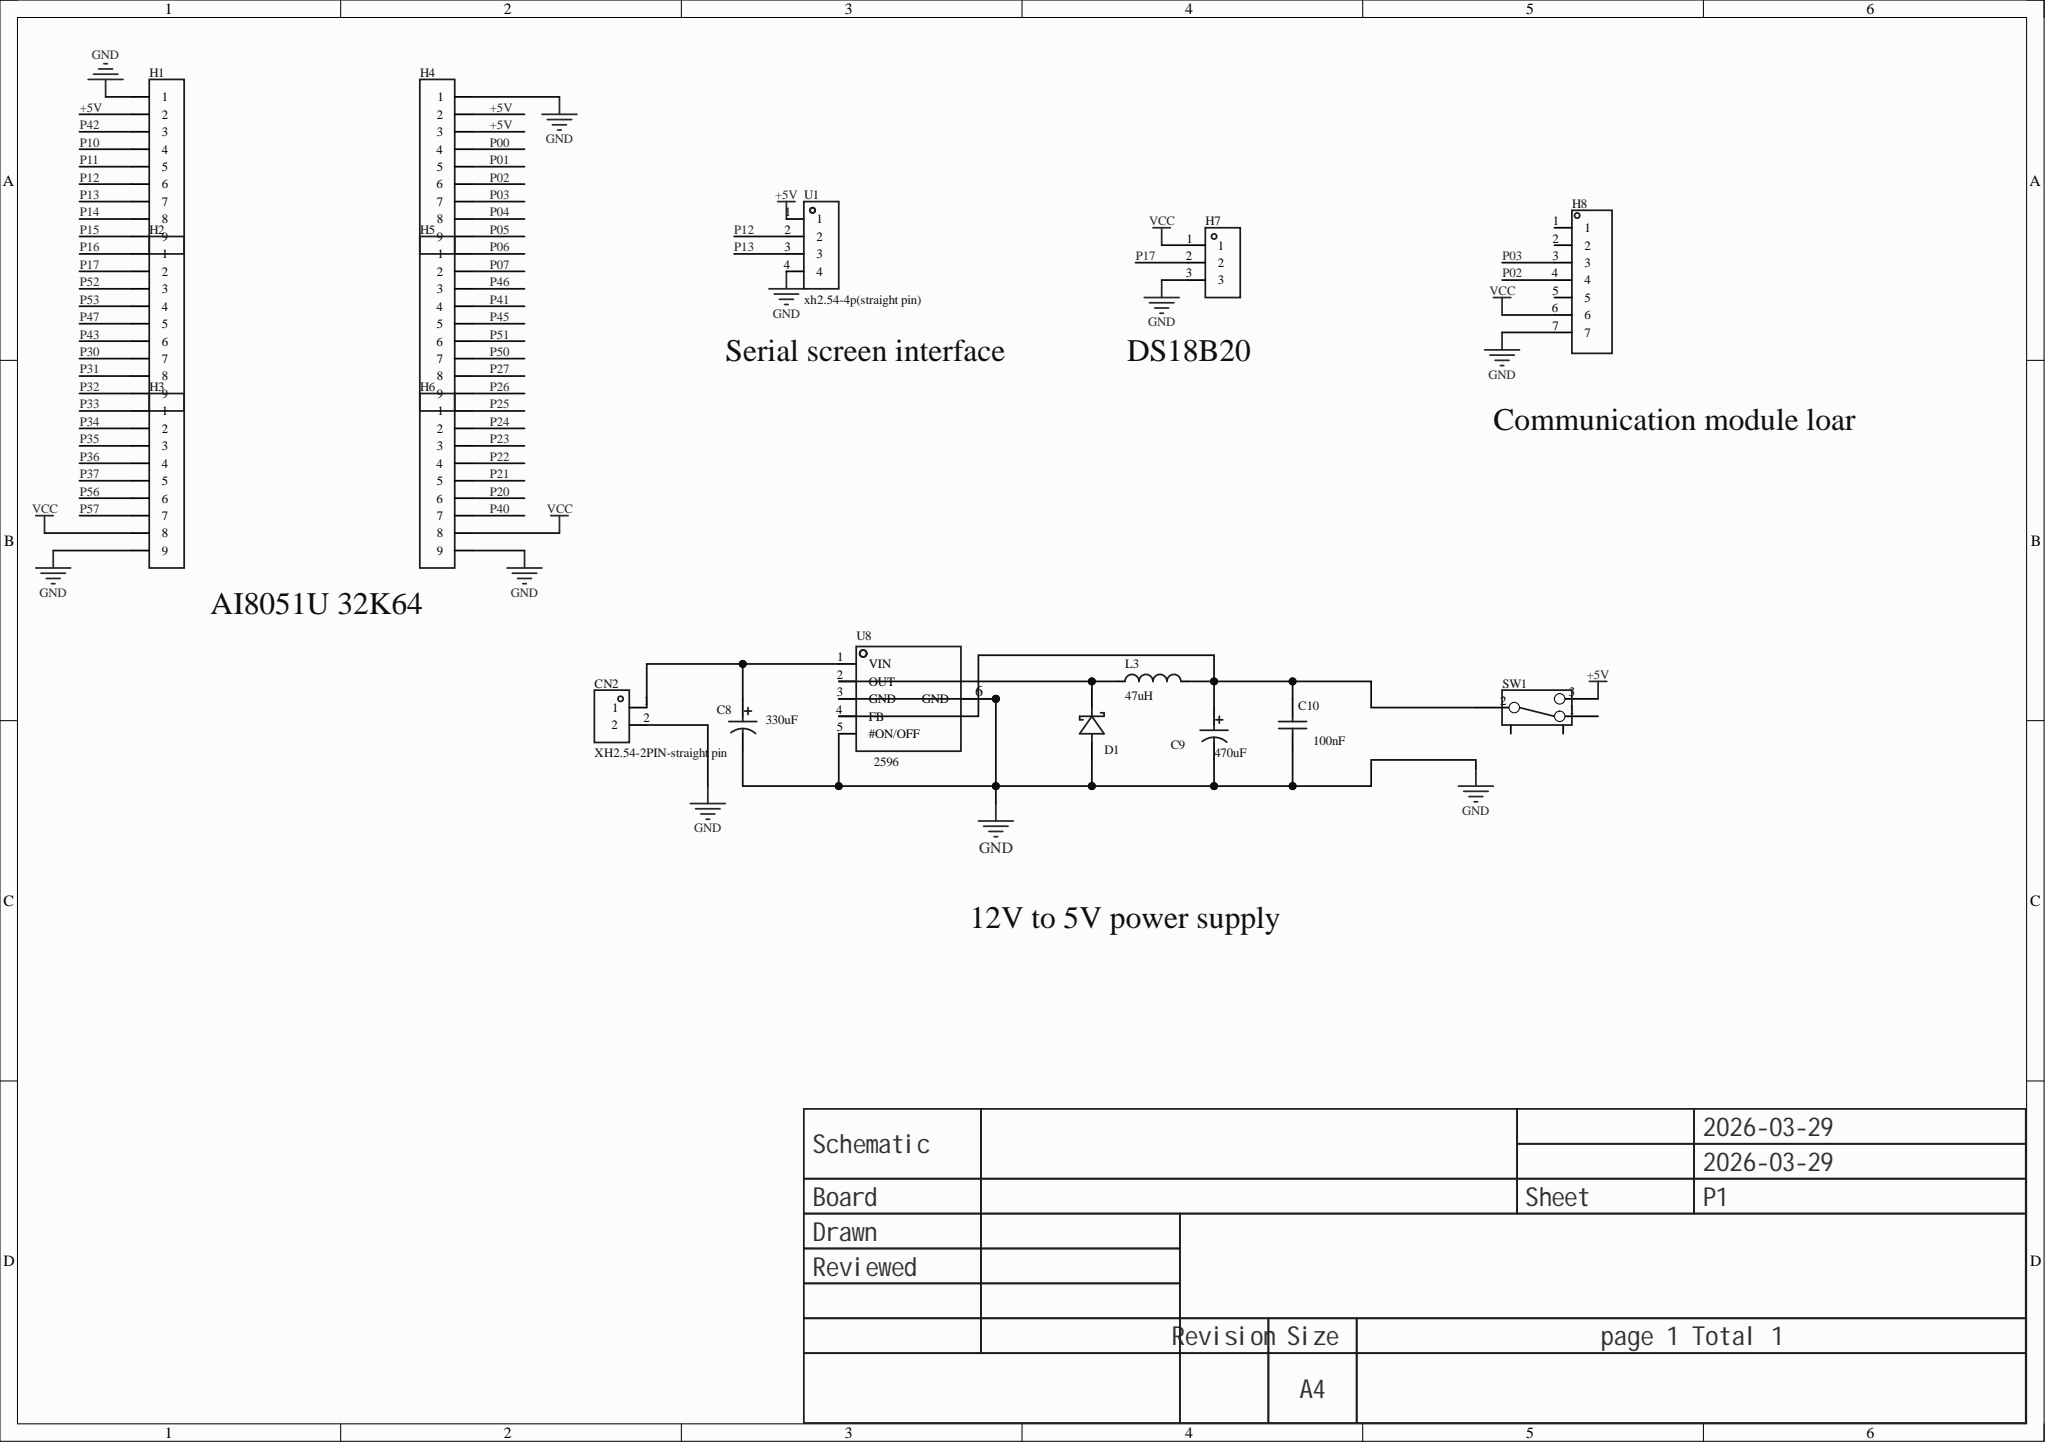Circuit board | Altium Designer | 17 parts | 11 nets
Bill of materials:
Comment,Description,Designator,Footprint,LibRef,Quantity
"","Capacitance: 220uF; tolerance: ±20%; rated voltage: 35V; body diameter: 8mm; body length: 10.5mm; ripple current: -; ESR: -; life: 2000hrs@105; operating temperature: -40~+105;","C8, C9","CAP-SMD_BD8.0-L8.3-W8.3-RD","CS1V221M-CRF10","2"
"","Capacitance: 100nF; tolerance: ±10%; rated voltage: 50V; temperature coefficient: X7R;","C10","C0805","CL21B104KBCNNNC","1"
"XH2.54-2PIN-straight pin","","CN2","CONN-TH_XH2.54-2P","XH2.54-2PIN-直针","1"
"","","D1","SMA_L4.3-W2.6-LS5.2-RD","SS34_3","1"
"","","H1, H2, H3, H4, H5, H6","HDR-TH_9P-P2.54-V-F-1","HDR-F_2.54_1x9P","6"
"","","H7","HDR-TH_3P-P2.54-V-F","HDR-F_2.54_1x3P","1"
"","","H8","HDR-TH_7P-P2.54-V-F","HDR-F_2.54_1x7P","1"
"","Inductance: 33uH; tolerance: ±20%; DC resistance (DCR): 270mO;","L3","IND-SMD_L7.0-W6.6","CMLO0630H330MTT","1"
"","","SW1","拨动开关","拨动开关_正","1"
"xh2.54-4p(straight pin)","","U1","CONN-TH_4P-P2.50-XH2.54-4P","xh2.54-4p(直针)","1"
"LM2596S-5.0","Function type: step-down; output type: fixed; input voltage: 40V; output voltage: 5V; output current (max): 3A;","U8","TO-263-5_L10.2-W8.9-P1.70-BR","LM2596S-5.0_C347421","1"
Netlist (Protel format):
[
C8
CAP-SMD_BD8.0-L8.3-W8.3-RD




]
[
C9
CAP-SMD_BD8.0-L8.3-W8.3-RD




]
[
C10
C0805




]
[
CN2
CONN-TH_XH2.54-2P
XH2.54-2PIN-straight pin



]
[
D1
SMA_L4.3-W2.6-LS5.2-RD




]
[
H1
HDR-TH_9P-P2.54-V-F-1




]
[
H2
HDR-TH_9P-P2.54-V-F-1




]
[
H3
HDR-TH_9P-P2.54-V-F-1




]
[
H4
HDR-TH_9P-P2.54-V-F-1




]
[
H5
HDR-TH_9P-P2.54-V-F-1




]
[
H6
HDR-TH_9P-P2.54-V-F-1




]
[
H7
HDR-TH_3P-P2.54-V-F




]
[
H8
HDR-TH_7P-P2.54-V-F




]
[
L3
IND-SMD_L7.0-W6.6




]
[
SW1
拨动开关




]
[
U1
CONN-TH_4P-P2.50-XH2.54-4P
xh2.54-4p(straight pin)



]
[
U8
TO-263-5_L10.2-W8.9-P1.70-BR
LM2596S-5.0



]
(
VCC
H3-8
H6-8
H7-1
H8-6
)
(
P17
H2-2
H7-2
)
(
P13
H1-7
U1-3
)
(
P12
H1-6
U1-2
)
(
P03
H4-7
H8-3
)
(
P02
H4-6
H8-4
)
(
NetD1_1
D1-1
L3-1
U8-2
)
(
NetC9_1
C9-1
C10-1
L3-2
SW1-2
U8-4
)
(
NetC8_1
C8-1
CN2-1
U8-1
)
(
GND
C8-2
C9-2
C10-2
CN2-2
D1-2
H1-1
H3-9
H4-1
H6-9
H7-3
H8-7
U1-4
U8-3
U8-5
U8-6
)
(
+5V
H1-2
H4-2
H4-3
SW1-3
U1-1
)